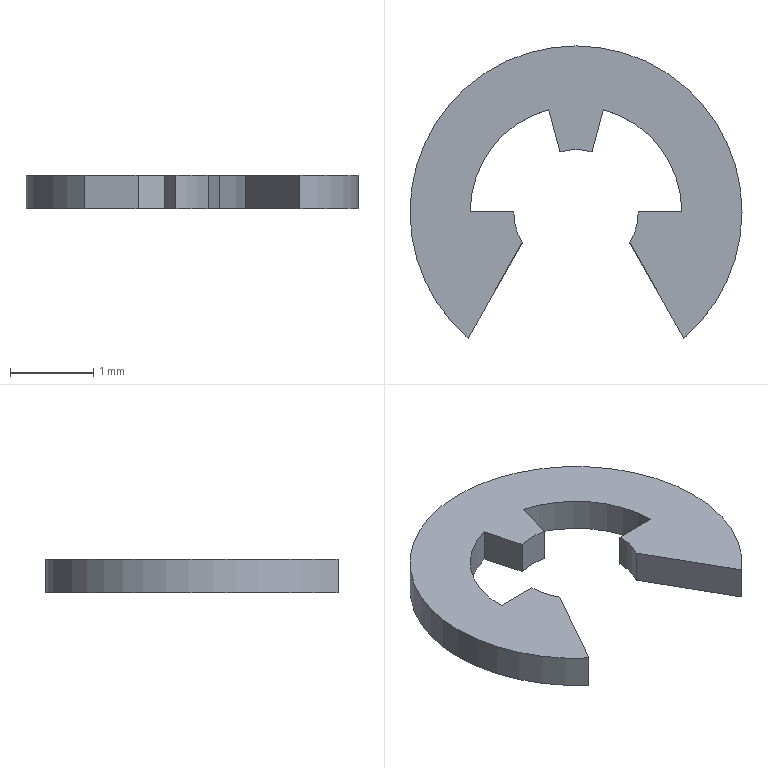Part | NX | 1 solid | 14 faces | box 4 x 3.52 x 0.4 mm | volume 2.666 mm3 | plane 8 | cylinder 6 | commonest cylinder face diameters 1.5 x3 2.55 x2 4 x1
STEP:
#1=CARTESIAN_POINT('',(1.3,-1.52,-0.2));
#2=VERTEX_POINT('',#1);
#3=CARTESIAN_POINT('',(-1.3,-1.52,-0.2));
#4=VERTEX_POINT('',#3);
#5=CARTESIAN_POINT('',(0.,0.,-0.2));
#6=DIRECTION('',(0.,0.,1.));
#7=DIRECTION('',(0.65,-0.7599,0.));
#8=AXIS2_PLACEMENT_3D('',#5,#6,#7);
#9=CIRCLE('',#8,2.);
#10=EDGE_CURVE('',#2,#4,#9,.T.);
#11=ORIENTED_EDGE('',*,*,#10,.T.);
#12=CARTESIAN_POINT('',(-1.3,-1.52,0.2));
#13=VERTEX_POINT('',#12);
#14=CARTESIAN_POINT('',(-1.3,-1.52,0.2));
#15=DIRECTION('',(0.,0.,-1.));
#16=VECTOR('',#15,1000.);
#17=LINE('',#14,#16);
#18=EDGE_CURVE('',#13,#4,#17,.T.);
#19=ORIENTED_EDGE('',*,*,#18,.F.);
#20=CARTESIAN_POINT('',(1.3,-1.52,0.2));
#21=VERTEX_POINT('',#20);
#22=CARTESIAN_POINT('',(0.,0.,0.2));
#23=DIRECTION('',(0.,0.,1.));
#24=DIRECTION('',(0.65,-0.7599,0.));
#25=AXIS2_PLACEMENT_3D('',#22,#23,#24);
#26=CIRCLE('',#25,2.);
#27=EDGE_CURVE('',#21,#13,#26,.T.);
#28=ORIENTED_EDGE('',*,*,#27,.F.);
#29=CARTESIAN_POINT('',(1.3,-1.52,0.2));
#30=DIRECTION('',(0.,0.,-1.));
#31=VECTOR('',#30,1000.);
#32=LINE('',#29,#31);
#33=EDGE_CURVE('',#21,#2,#32,.T.);
#34=ORIENTED_EDGE('',*,*,#33,.T.);
#35=EDGE_LOOP('',(#11,#19,#28,#34));
#36=FACE_BOUND('',#35,.T.);
#37=CARTESIAN_POINT('',(0.,0.,0.2));
#38=DIRECTION('',(0.,0.,1.));
#39=DIRECTION('',(0.65,-0.7599,0.));
#40=AXIS2_PLACEMENT_3D('',#37,#38,#39);
#41=CYLINDRICAL_SURFACE('',#40,2.);
#42=ADVANCED_FACE('',(#36),#41,.T.);
#43=CARTESIAN_POINT('',(-0.65,-0.3742,-0.2));
#44=VERTEX_POINT('',#43);
#45=CARTESIAN_POINT('',(-1.3,-1.52,-0.2));
#46=DIRECTION('',(0.4935,0.8698,0.));
#47=VECTOR('',#46,1000.);
#48=LINE('',#45,#47);
#49=EDGE_CURVE('',#4,#44,#48,.T.);
#50=ORIENTED_EDGE('',*,*,#49,.T.);
#51=CARTESIAN_POINT('',(-0.65,-0.3742,0.2));
#52=VERTEX_POINT('',#51);
#53=CARTESIAN_POINT('',(-0.65,-0.3742,0.2));
#54=DIRECTION('',(0.,0.,-1.));
#55=VECTOR('',#54,1000.);
#56=LINE('',#53,#55);
#57=EDGE_CURVE('',#52,#44,#56,.T.);
#58=ORIENTED_EDGE('',*,*,#57,.F.);
#59=CARTESIAN_POINT('',(-1.3,-1.52,0.2));
#60=DIRECTION('',(0.4935,0.8698,0.));
#61=VECTOR('',#60,1000.);
#62=LINE('',#59,#61);
#63=EDGE_CURVE('',#13,#52,#62,.T.);
#64=ORIENTED_EDGE('',*,*,#63,.F.);
#65=ORIENTED_EDGE('',*,*,#18,.T.);
#66=EDGE_LOOP('',(#50,#58,#64,#65));
#67=FACE_BOUND('',#66,.T.);
#68=CARTESIAN_POINT('',(-1.3,-1.52,0.2));
#69=DIRECTION('',(0.8698,-0.4935,0.));
#70=DIRECTION('',(0.,0.,-1.));
#71=AXIS2_PLACEMENT_3D('',#68,#69,#70);
#72=PLANE('',#71);
#73=ADVANCED_FACE('',(#67),#72,.T.);
#74=CARTESIAN_POINT('',(-0.75,0.,-0.2));
#75=VERTEX_POINT('',#74);
#76=CARTESIAN_POINT('',(0.,0.,-0.2));
#77=DIRECTION('',(0.,0.,-1.));
#78=DIRECTION('',(-0.8667,-0.4989,0.));
#79=AXIS2_PLACEMENT_3D('',#76,#77,#78);
#80=CIRCLE('',#79,0.75);
#81=EDGE_CURVE('',#44,#75,#80,.T.);
#82=ORIENTED_EDGE('',*,*,#81,.T.);
#83=CARTESIAN_POINT('',(-0.75,0.,0.2));
#84=VERTEX_POINT('',#83);
#85=CARTESIAN_POINT('',(-0.75,0.,0.2));
#86=DIRECTION('',(0.,0.,-1.));
#87=VECTOR('',#86,1000.);
#88=LINE('',#85,#87);
#89=EDGE_CURVE('',#84,#75,#88,.T.);
#90=ORIENTED_EDGE('',*,*,#89,.F.);
#91=CARTESIAN_POINT('',(0.,0.,0.2));
#92=DIRECTION('',(0.,0.,-1.));
#93=DIRECTION('',(-0.8667,-0.4989,0.));
#94=AXIS2_PLACEMENT_3D('',#91,#92,#93);
#95=CIRCLE('',#94,0.75);
#96=EDGE_CURVE('',#52,#84,#95,.T.);
#97=ORIENTED_EDGE('',*,*,#96,.F.);
#98=ORIENTED_EDGE('',*,*,#57,.T.);
#99=EDGE_LOOP('',(#82,#90,#97,#98));
#100=FACE_BOUND('',#99,.T.);
#101=CARTESIAN_POINT('',(0.,0.,0.2));
#102=DIRECTION('',(0.,0.,1.));
#103=DIRECTION('',(-0.8667,-0.4989,0.));
#104=AXIS2_PLACEMENT_3D('',#101,#102,#103);
#105=CYLINDRICAL_SURFACE('',#104,0.75);
#106=ADVANCED_FACE('',(#100),#105,.F.);
#107=CARTESIAN_POINT('',(-1.275,0.,-0.2));
#108=VERTEX_POINT('',#107);
#109=CARTESIAN_POINT('',(-0.75,0.,-0.2));
#110=DIRECTION('',(-1.,0.,0.));
#111=VECTOR('',#110,1000.);
#112=LINE('',#109,#111);
#113=EDGE_CURVE('',#75,#108,#112,.T.);
#114=ORIENTED_EDGE('',*,*,#113,.T.);
#115=CARTESIAN_POINT('',(-1.275,0.,0.2));
#116=VERTEX_POINT('',#115);
#117=CARTESIAN_POINT('',(-1.275,0.,0.2));
#118=DIRECTION('',(0.,0.,-1.));
#119=VECTOR('',#118,1000.);
#120=LINE('',#117,#119);
#121=EDGE_CURVE('',#116,#108,#120,.T.);
#122=ORIENTED_EDGE('',*,*,#121,.F.);
#123=CARTESIAN_POINT('',(-0.75,0.,0.2));
#124=DIRECTION('',(-1.,0.,0.));
#125=VECTOR('',#124,1000.);
#126=LINE('',#123,#125);
#127=EDGE_CURVE('',#84,#116,#126,.T.);
#128=ORIENTED_EDGE('',*,*,#127,.F.);
#129=ORIENTED_EDGE('',*,*,#89,.T.);
#130=EDGE_LOOP('',(#114,#122,#128,#129));
#131=FACE_BOUND('',#130,.T.);
#132=CARTESIAN_POINT('',(-0.75,0.,0.2));
#133=DIRECTION('',(0.,1.,0.));
#134=DIRECTION('',(1.,0.,0.));
#135=AXIS2_PLACEMENT_3D('',#132,#133,#134);
#136=PLANE('',#135);
#137=ADVANCED_FACE('',(#131),#136,.T.);
#138=CARTESIAN_POINT('',(-0.33,1.232,-0.2));
#139=VERTEX_POINT('',#138);
#140=CARTESIAN_POINT('',(0.,0.,-0.2));
#141=DIRECTION('',(0.,0.,-1.));
#142=DIRECTION('',(-1.,0.,0.));
#143=AXIS2_PLACEMENT_3D('',#140,#141,#142);
#144=CIRCLE('',#143,1.275);
#145=EDGE_CURVE('',#108,#139,#144,.T.);
#146=ORIENTED_EDGE('',*,*,#145,.T.);
#147=CARTESIAN_POINT('',(-0.33,1.232,0.2));
#148=VERTEX_POINT('',#147);
#149=CARTESIAN_POINT('',(-0.33,1.232,0.2));
#150=DIRECTION('',(0.,0.,-1.));
#151=VECTOR('',#150,1000.);
#152=LINE('',#149,#151);
#153=EDGE_CURVE('',#148,#139,#152,.T.);
#154=ORIENTED_EDGE('',*,*,#153,.F.);
#155=CARTESIAN_POINT('',(0.,0.,0.2));
#156=DIRECTION('',(0.,0.,-1.));
#157=DIRECTION('',(-1.,0.,0.));
#158=AXIS2_PLACEMENT_3D('',#155,#156,#157);
#159=CIRCLE('',#158,1.275);
#160=EDGE_CURVE('',#116,#148,#159,.T.);
#161=ORIENTED_EDGE('',*,*,#160,.F.);
#162=ORIENTED_EDGE('',*,*,#121,.T.);
#163=EDGE_LOOP('',(#146,#154,#161,#162));
#164=FACE_BOUND('',#163,.T.);
#165=CARTESIAN_POINT('',(0.,0.,0.2));
#166=DIRECTION('',(0.,0.,1.));
#167=DIRECTION('',(-1.,0.,0.));
#168=AXIS2_PLACEMENT_3D('',#165,#166,#167);
#169=CYLINDRICAL_SURFACE('',#168,1.275);
#170=ADVANCED_FACE('',(#164),#169,.F.);
#171=CARTESIAN_POINT('',(-0.1941,0.7244,-0.2));
#172=VERTEX_POINT('',#171);
#173=CARTESIAN_POINT('',(-0.33,1.232,-0.2));
#174=DIRECTION('',(0.2588,-0.9659,0.));
#175=VECTOR('',#174,1000.);
#176=LINE('',#173,#175);
#177=EDGE_CURVE('',#139,#172,#176,.T.);
#178=ORIENTED_EDGE('',*,*,#177,.T.);
#179=CARTESIAN_POINT('',(-0.1941,0.7244,0.2));
#180=VERTEX_POINT('',#179);
#181=CARTESIAN_POINT('',(-0.1941,0.7244,0.2));
#182=DIRECTION('',(0.,0.,-1.));
#183=VECTOR('',#182,1000.);
#184=LINE('',#181,#183);
#185=EDGE_CURVE('',#180,#172,#184,.T.);
#186=ORIENTED_EDGE('',*,*,#185,.F.);
#187=CARTESIAN_POINT('',(-0.33,1.232,0.2));
#188=DIRECTION('',(0.2588,-0.9659,0.));
#189=VECTOR('',#188,1000.);
#190=LINE('',#187,#189);
#191=EDGE_CURVE('',#148,#180,#190,.T.);
#192=ORIENTED_EDGE('',*,*,#191,.F.);
#193=ORIENTED_EDGE('',*,*,#153,.T.);
#194=EDGE_LOOP('',(#178,#186,#192,#193));
#195=FACE_BOUND('',#194,.T.);
#196=CARTESIAN_POINT('',(-0.33,1.232,0.2));
#197=DIRECTION('',(-0.9659,-0.2588,0.));
#198=DIRECTION('',(-0.2588,0.9659,0.));
#199=AXIS2_PLACEMENT_3D('',#196,#197,#198);
#200=PLANE('',#199);
#201=ADVANCED_FACE('',(#195),#200,.T.);
#202=CARTESIAN_POINT('',(0.1941,0.7244,-0.2));
#203=VERTEX_POINT('',#202);
#204=CARTESIAN_POINT('',(0.,0.,-0.2));
#205=DIRECTION('',(0.,0.,-1.));
#206=DIRECTION('',(-0.2588,0.9659,0.));
#207=AXIS2_PLACEMENT_3D('',#204,#205,#206);
#208=CIRCLE('',#207,0.75);
#209=EDGE_CURVE('',#172,#203,#208,.T.);
#210=ORIENTED_EDGE('',*,*,#209,.T.);
#211=CARTESIAN_POINT('',(0.1941,0.7244,0.2));
#212=VERTEX_POINT('',#211);
#213=CARTESIAN_POINT('',(0.1941,0.7244,0.2));
#214=DIRECTION('',(0.,0.,-1.));
#215=VECTOR('',#214,1000.);
#216=LINE('',#213,#215);
#217=EDGE_CURVE('',#212,#203,#216,.T.);
#218=ORIENTED_EDGE('',*,*,#217,.F.);
#219=CARTESIAN_POINT('',(0.,0.,0.2));
#220=DIRECTION('',(0.,0.,-1.));
#221=DIRECTION('',(-0.2588,0.9659,0.));
#222=AXIS2_PLACEMENT_3D('',#219,#220,#221);
#223=CIRCLE('',#222,0.75);
#224=EDGE_CURVE('',#180,#212,#223,.T.);
#225=ORIENTED_EDGE('',*,*,#224,.F.);
#226=ORIENTED_EDGE('',*,*,#185,.T.);
#227=EDGE_LOOP('',(#210,#218,#225,#226));
#228=FACE_BOUND('',#227,.T.);
#229=CARTESIAN_POINT('',(0.,0.,0.2));
#230=DIRECTION('',(0.,0.,1.));
#231=DIRECTION('',(-0.2588,0.9659,0.));
#232=AXIS2_PLACEMENT_3D('',#229,#230,#231);
#233=CYLINDRICAL_SURFACE('',#232,0.75);
#234=ADVANCED_FACE('',(#228),#233,.F.);
#235=CARTESIAN_POINT('',(0.33,1.232,-0.2));
#236=VERTEX_POINT('',#235);
#237=CARTESIAN_POINT('',(0.1941,0.7244,-0.2));
#238=DIRECTION('',(0.2588,0.9659,0.));
#239=VECTOR('',#238,1000.);
#240=LINE('',#237,#239);
#241=EDGE_CURVE('',#203,#236,#240,.T.);
#242=ORIENTED_EDGE('',*,*,#241,.T.);
#243=CARTESIAN_POINT('',(0.33,1.232,0.2));
#244=VERTEX_POINT('',#243);
#245=CARTESIAN_POINT('',(0.33,1.232,0.2));
#246=DIRECTION('',(0.,0.,-1.));
#247=VECTOR('',#246,1000.);
#248=LINE('',#245,#247);
#249=EDGE_CURVE('',#244,#236,#248,.T.);
#250=ORIENTED_EDGE('',*,*,#249,.F.);
#251=CARTESIAN_POINT('',(0.1941,0.7244,0.2));
#252=DIRECTION('',(0.2588,0.9659,0.));
#253=VECTOR('',#252,1000.);
#254=LINE('',#251,#253);
#255=EDGE_CURVE('',#212,#244,#254,.T.);
#256=ORIENTED_EDGE('',*,*,#255,.F.);
#257=ORIENTED_EDGE('',*,*,#217,.T.);
#258=EDGE_LOOP('',(#242,#250,#256,#257));
#259=FACE_BOUND('',#258,.T.);
#260=CARTESIAN_POINT('',(0.1941,0.7244,0.2));
#261=DIRECTION('',(0.9659,-0.2588,0.));
#262=DIRECTION('',(0.,0.,-1.));
#263=AXIS2_PLACEMENT_3D('',#260,#261,#262);
#264=PLANE('',#263);
#265=ADVANCED_FACE('',(#259),#264,.T.);
#266=CARTESIAN_POINT('',(1.275,0.,-0.2));
#267=VERTEX_POINT('',#266);
#268=CARTESIAN_POINT('',(0.,0.,-0.2));
#269=DIRECTION('',(0.,0.,-1.));
#270=DIRECTION('',(0.2588,0.9659,0.));
#271=AXIS2_PLACEMENT_3D('',#268,#269,#270);
#272=CIRCLE('',#271,1.275);
#273=EDGE_CURVE('',#236,#267,#272,.T.);
#274=ORIENTED_EDGE('',*,*,#273,.T.);
#275=CARTESIAN_POINT('',(1.275,0.,0.2));
#276=VERTEX_POINT('',#275);
#277=CARTESIAN_POINT('',(1.275,0.,0.2));
#278=DIRECTION('',(0.,0.,-1.));
#279=VECTOR('',#278,1000.);
#280=LINE('',#277,#279);
#281=EDGE_CURVE('',#276,#267,#280,.T.);
#282=ORIENTED_EDGE('',*,*,#281,.F.);
#283=CARTESIAN_POINT('',(0.,0.,0.2));
#284=DIRECTION('',(0.,0.,-1.));
#285=DIRECTION('',(0.2588,0.9659,0.));
#286=AXIS2_PLACEMENT_3D('',#283,#284,#285);
#287=CIRCLE('',#286,1.275);
#288=EDGE_CURVE('',#244,#276,#287,.T.);
#289=ORIENTED_EDGE('',*,*,#288,.F.);
#290=ORIENTED_EDGE('',*,*,#249,.T.);
#291=EDGE_LOOP('',(#274,#282,#289,#290));
#292=FACE_BOUND('',#291,.T.);
#293=CARTESIAN_POINT('',(0.,0.,0.2));
#294=DIRECTION('',(0.,0.,1.));
#295=DIRECTION('',(0.2588,0.9659,0.));
#296=AXIS2_PLACEMENT_3D('',#293,#294,#295);
#297=CYLINDRICAL_SURFACE('',#296,1.275);
#298=ADVANCED_FACE('',(#292),#297,.F.);
#299=CARTESIAN_POINT('',(0.75,0.,-0.2));
#300=VERTEX_POINT('',#299);
#301=CARTESIAN_POINT('',(1.275,0.,-0.2));
#302=DIRECTION('',(-1.,0.,0.));
#303=VECTOR('',#302,1000.);
#304=LINE('',#301,#303);
#305=EDGE_CURVE('',#267,#300,#304,.T.);
#306=ORIENTED_EDGE('',*,*,#305,.T.);
#307=CARTESIAN_POINT('',(0.75,0.,0.2));
#308=VERTEX_POINT('',#307);
#309=CARTESIAN_POINT('',(0.75,0.,0.2));
#310=DIRECTION('',(0.,0.,-1.));
#311=VECTOR('',#310,1000.);
#312=LINE('',#309,#311);
#313=EDGE_CURVE('',#308,#300,#312,.T.);
#314=ORIENTED_EDGE('',*,*,#313,.F.);
#315=CARTESIAN_POINT('',(1.275,0.,0.2));
#316=DIRECTION('',(-1.,0.,0.));
#317=VECTOR('',#316,1000.);
#318=LINE('',#315,#317);
#319=EDGE_CURVE('',#276,#308,#318,.T.);
#320=ORIENTED_EDGE('',*,*,#319,.F.);
#321=ORIENTED_EDGE('',*,*,#281,.T.);
#322=EDGE_LOOP('',(#306,#314,#320,#321));
#323=FACE_BOUND('',#322,.T.);
#324=CARTESIAN_POINT('',(1.275,0.,0.2));
#325=DIRECTION('',(0.,1.,0.));
#326=DIRECTION('',(1.,0.,0.));
#327=AXIS2_PLACEMENT_3D('',#324,#325,#326);
#328=PLANE('',#327);
#329=ADVANCED_FACE('',(#323),#328,.T.);
#330=CARTESIAN_POINT('',(0.65,-0.3742,-0.2));
#331=VERTEX_POINT('',#330);
#332=CARTESIAN_POINT('',(0.,0.,-0.2));
#333=DIRECTION('',(0.,0.,-1.));
#334=DIRECTION('',(1.,0.,0.));
#335=AXIS2_PLACEMENT_3D('',#332,#333,#334);
#336=CIRCLE('',#335,0.75);
#337=EDGE_CURVE('',#300,#331,#336,.T.);
#338=ORIENTED_EDGE('',*,*,#337,.T.);
#339=CARTESIAN_POINT('',(0.65,-0.3742,0.2));
#340=VERTEX_POINT('',#339);
#341=CARTESIAN_POINT('',(0.65,-0.3742,0.2));
#342=DIRECTION('',(0.,0.,-1.));
#343=VECTOR('',#342,1000.);
#344=LINE('',#341,#343);
#345=EDGE_CURVE('',#340,#331,#344,.T.);
#346=ORIENTED_EDGE('',*,*,#345,.F.);
#347=CARTESIAN_POINT('',(0.,0.,0.2));
#348=DIRECTION('',(0.,0.,-1.));
#349=DIRECTION('',(1.,0.,0.));
#350=AXIS2_PLACEMENT_3D('',#347,#348,#349);
#351=CIRCLE('',#350,0.75);
#352=EDGE_CURVE('',#308,#340,#351,.T.);
#353=ORIENTED_EDGE('',*,*,#352,.F.);
#354=ORIENTED_EDGE('',*,*,#313,.T.);
#355=EDGE_LOOP('',(#338,#346,#353,#354));
#356=FACE_BOUND('',#355,.T.);
#357=CARTESIAN_POINT('',(0.,0.,0.2));
#358=DIRECTION('',(0.,0.,1.));
#359=DIRECTION('',(1.,0.,0.));
#360=AXIS2_PLACEMENT_3D('',#357,#358,#359);
#361=CYLINDRICAL_SURFACE('',#360,0.75);
#362=ADVANCED_FACE('',(#356),#361,.F.);
#363=CARTESIAN_POINT('',(0.65,-0.3742,-0.2));
#364=DIRECTION('',(0.4935,-0.8698,0.));
#365=VECTOR('',#364,1000.);
#366=LINE('',#363,#365);
#367=EDGE_CURVE('',#331,#2,#366,.T.);
#368=ORIENTED_EDGE('',*,*,#367,.T.);
#369=ORIENTED_EDGE('',*,*,#33,.F.);
#370=CARTESIAN_POINT('',(0.65,-0.3742,0.2));
#371=DIRECTION('',(0.4935,-0.8698,0.));
#372=VECTOR('',#371,1000.);
#373=LINE('',#370,#372);
#374=EDGE_CURVE('',#340,#21,#373,.T.);
#375=ORIENTED_EDGE('',*,*,#374,.F.);
#376=ORIENTED_EDGE('',*,*,#345,.T.);
#377=EDGE_LOOP('',(#368,#369,#375,#376));
#378=FACE_BOUND('',#377,.T.);
#379=CARTESIAN_POINT('',(0.65,-0.3742,0.2));
#380=DIRECTION('',(-0.8698,-0.4935,0.));
#381=DIRECTION('',(-0.4935,0.8698,0.));
#382=AXIS2_PLACEMENT_3D('',#379,#380,#381);
#383=PLANE('',#382);
#384=ADVANCED_FACE('',(#378),#383,.T.);
#385=ORIENTED_EDGE('',*,*,#27,.T.);
#386=ORIENTED_EDGE('',*,*,#63,.T.);
#387=ORIENTED_EDGE('',*,*,#96,.T.);
#388=ORIENTED_EDGE('',*,*,#127,.T.);
#389=ORIENTED_EDGE('',*,*,#160,.T.);
#390=ORIENTED_EDGE('',*,*,#191,.T.);
#391=ORIENTED_EDGE('',*,*,#224,.T.);
#392=ORIENTED_EDGE('',*,*,#255,.T.);
#393=ORIENTED_EDGE('',*,*,#288,.T.);
#394=ORIENTED_EDGE('',*,*,#319,.T.);
#395=ORIENTED_EDGE('',*,*,#352,.T.);
#396=ORIENTED_EDGE('',*,*,#374,.T.);
#397=EDGE_LOOP('',(#385,#386,#387,#388,#389,#390,#391,#392,#393,#394,#395,#396));
#398=FACE_BOUND('',#397,.T.);
#399=CARTESIAN_POINT('',(0.,0.,0.2));
#400=DIRECTION('',(0.,0.,1.));
#401=DIRECTION('',(1.,0.,0.));
#402=AXIS2_PLACEMENT_3D('',#399,#400,#401);
#403=PLANE('',#402);
#404=ADVANCED_FACE('',(#398),#403,.T.);
#405=ORIENTED_EDGE('',*,*,#49,.F.);
#406=ORIENTED_EDGE('',*,*,#10,.F.);
#407=ORIENTED_EDGE('',*,*,#367,.F.);
#408=ORIENTED_EDGE('',*,*,#337,.F.);
#409=ORIENTED_EDGE('',*,*,#305,.F.);
#410=ORIENTED_EDGE('',*,*,#273,.F.);
#411=ORIENTED_EDGE('',*,*,#241,.F.);
#412=ORIENTED_EDGE('',*,*,#209,.F.);
#413=ORIENTED_EDGE('',*,*,#177,.F.);
#414=ORIENTED_EDGE('',*,*,#145,.F.);
#415=ORIENTED_EDGE('',*,*,#113,.F.);
#416=ORIENTED_EDGE('',*,*,#81,.F.);
#417=EDGE_LOOP('',(#405,#406,#407,#408,#409,#410,#411,#412,#413,#414,#415,#416));
#418=FACE_BOUND('',#417,.T.);
#419=CARTESIAN_POINT('',(0.,0.,-0.2));
#420=DIRECTION('',(0.,0.,1.));
#421=DIRECTION('',(1.,0.,0.));
#422=AXIS2_PLACEMENT_3D('',#419,#420,#421);
#423=PLANE('',#422);
#424=ADVANCED_FACE('',(#418),#423,.F.);
#425=CLOSED_SHELL('',(#42,#73,#106,#137,#170,#201,#234,#265,#298,#329,#362,#384,#404,#424));
#426=MANIFOLD_SOLID_BREP('',#425);
#427=(LENGTH_UNIT()NAMED_UNIT(*)SI_UNIT(.MILLI.,.METRE.));
#428=UNCERTAINTY_MEASURE_WITH_UNIT(LENGTH_MEASURE(0.00001),#427,'','');
#429=(NAMED_UNIT(*)PLANE_ANGLE_UNIT()SI_UNIT($,.RADIAN.));
#430=(NAMED_UNIT(*)SI_UNIT($,.STERADIAN.)SOLID_ANGLE_UNIT());
#431=(GEOMETRIC_REPRESENTATION_CONTEXT(3)GLOBAL_UNCERTAINTY_ASSIGNED_CONTEXT((#428))GLOBAL_UNIT_ASSIGNED_CONTEXT((#427,#429,#430))REPRESENTATION_CONTEXT('',''));
#432=ADVANCED_BREP_SHAPE_REPRESENTATION('',(#426),#431);